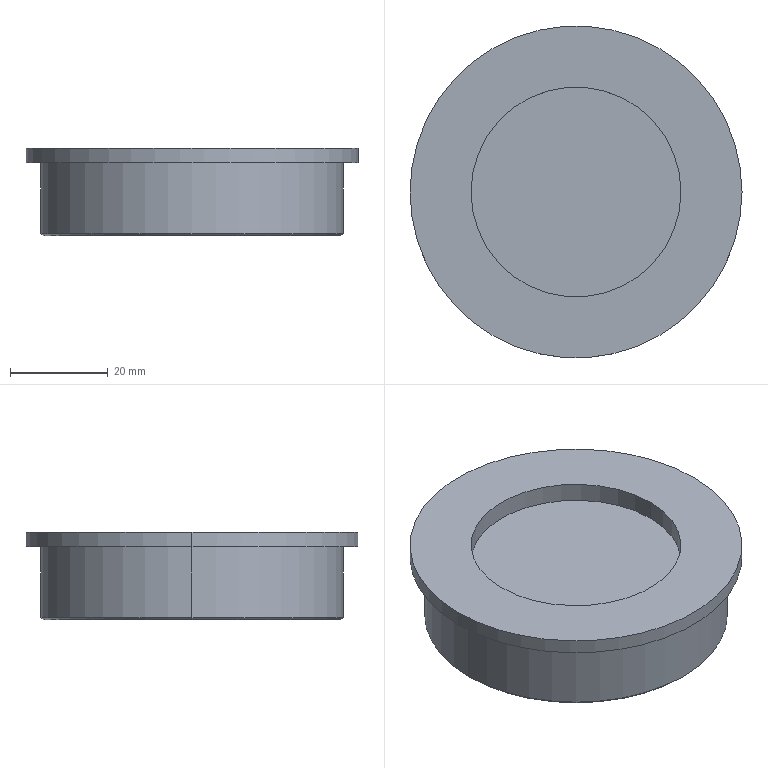Part | SolidWorks | features MBimport 1 | 1 solid | 12 faces | box 68 x 68 x 18 mm | volume 50348 mm3 | cylinder 6 | plane 4 | cone 2 | commonest cylinder face diameters 43 x2 62 x2 68 x2
STEP:
#1=CARTESIAN_POINT('',(-30.5,0.,0.));
#2=VERTEX_POINT('',#1);
#3=CARTESIAN_POINT('',(30.5,0.,0.));
#4=VERTEX_POINT('',#3);
#5=CARTESIAN_POINT('',(0.,0.,0.));
#6=DIRECTION('',(0.,0.,-1.));
#7=DIRECTION('',(-1.,0.,0.));
#8=AXIS2_PLACEMENT_3D('',#5,#6,#7);
#9=CIRCLE('',#8,30.5);
#10=EDGE_CURVE('',#2,#4,#9,.T.);
#11=ORIENTED_EDGE('',*,*,#10,.F.);
#12=CARTESIAN_POINT('',(-31.,0.,0.5));
#13=VERTEX_POINT('',#12);
#14=CARTESIAN_POINT('',(-31.,0.,0.5));
#15=DIRECTION('',(-0.7071,0.,0.7071));
#16=VECTOR('',#15,1000.);
#17=LINE('',#14,#16);
#18=EDGE_CURVE('',#2,#13,#17,.T.);
#19=ORIENTED_EDGE('',*,*,#18,.T.);
#20=CARTESIAN_POINT('',(31.,0.,0.5));
#21=VERTEX_POINT('',#20);
#22=CARTESIAN_POINT('',(0.,0.,0.5));
#23=DIRECTION('',(0.,0.,1.));
#24=DIRECTION('',(-1.,0.,0.));
#25=AXIS2_PLACEMENT_3D('',#22,#23,#24);
#26=CIRCLE('',#25,31.);
#27=EDGE_CURVE('',#21,#13,#26,.T.);
#28=ORIENTED_EDGE('',*,*,#27,.F.);
#29=CARTESIAN_POINT('',(31.,0.,0.5));
#30=DIRECTION('',(0.7071,0.,0.7071));
#31=VECTOR('',#30,1000.);
#32=LINE('',#29,#31);
#33=EDGE_CURVE('',#4,#21,#32,.T.);
#34=ORIENTED_EDGE('',*,*,#33,.F.);
#35=EDGE_LOOP('',(#11,#19,#28,#34));
#36=FACE_OUTER_BOUND('',#35,.T.);
#37=CARTESIAN_POINT('',(0.,0.,0.5));
#38=DIRECTION('',(0.,0.,1.));
#39=DIRECTION('',(1.,0.,0.));
#40=AXIS2_PLACEMENT_3D('',#37,#38,#39);
#41=CONICAL_SURFACE('',#40,31.,0.7854);
#42=ADVANCED_FACE('',(#36),#41,.T.);
#43=CARTESIAN_POINT('',(21.5,0.,14.));
#44=VERTEX_POINT('',#43);
#45=CARTESIAN_POINT('',(-21.5,0.,14.));
#46=VERTEX_POINT('',#45);
#47=CARTESIAN_POINT('',(0.,0.,14.));
#48=DIRECTION('',(0.,0.,-1.));
#49=DIRECTION('',(1.,0.,0.));
#50=AXIS2_PLACEMENT_3D('',#47,#48,#49);
#51=CIRCLE('',#50,21.5);
#52=EDGE_CURVE('',#44,#46,#51,.T.);
#53=ORIENTED_EDGE('',*,*,#52,.T.);
#54=CARTESIAN_POINT('',(-21.5,0.,18.));
#55=VERTEX_POINT('',#54);
#56=CARTESIAN_POINT('',(-21.5,0.,14.));
#57=DIRECTION('',(0.,0.,1.));
#58=VECTOR('',#57,1000.);
#59=LINE('',#56,#58);
#60=EDGE_CURVE('',#46,#55,#59,.T.);
#61=ORIENTED_EDGE('',*,*,#60,.T.);
#62=CARTESIAN_POINT('',(21.5,0.,18.));
#63=VERTEX_POINT('',#62);
#64=CARTESIAN_POINT('',(0.,0.,18.));
#65=DIRECTION('',(0.,0.,1.));
#66=DIRECTION('',(1.,0.,0.));
#67=AXIS2_PLACEMENT_3D('',#64,#65,#66);
#68=CIRCLE('',#67,21.5);
#69=EDGE_CURVE('',#55,#63,#68,.T.);
#70=ORIENTED_EDGE('',*,*,#69,.T.);
#71=CARTESIAN_POINT('',(21.5,0.,14.));
#72=DIRECTION('',(0.,0.,1.));
#73=VECTOR('',#72,1000.);
#74=LINE('',#71,#73);
#75=EDGE_CURVE('',#44,#63,#74,.T.);
#76=ORIENTED_EDGE('',*,*,#75,.F.);
#77=EDGE_LOOP('',(#53,#61,#70,#76));
#78=FACE_OUTER_BOUND('',#77,.T.);
#79=CARTESIAN_POINT('',(0.,0.,14.));
#80=DIRECTION('',(0.,0.,1.));
#81=DIRECTION('',(1.,0.,0.));
#82=AXIS2_PLACEMENT_3D('',#79,#80,#81);
#83=CYLINDRICAL_SURFACE('',#82,21.5);
#84=ADVANCED_FACE('',(#78),#83,.F.);
#85=CARTESIAN_POINT('',(34.,0.,15.));
#86=VERTEX_POINT('',#85);
#87=CARTESIAN_POINT('',(-34.,0.,15.));
#88=VERTEX_POINT('',#87);
#89=CARTESIAN_POINT('',(0.,0.,15.));
#90=DIRECTION('',(0.,0.,1.));
#91=DIRECTION('',(1.,0.,0.));
#92=AXIS2_PLACEMENT_3D('',#89,#90,#91);
#93=CIRCLE('',#92,34.);
#94=EDGE_CURVE('',#86,#88,#93,.T.);
#95=ORIENTED_EDGE('',*,*,#94,.T.);
#96=CARTESIAN_POINT('',(-34.,0.,18.));
#97=VERTEX_POINT('',#96);
#98=CARTESIAN_POINT('',(-34.,0.,15.));
#99=DIRECTION('',(0.,0.,1.));
#100=VECTOR('',#99,1000.);
#101=LINE('',#98,#100);
#102=EDGE_CURVE('',#88,#97,#101,.T.);
#103=ORIENTED_EDGE('',*,*,#102,.T.);
#104=CARTESIAN_POINT('',(34.,0.,18.));
#105=VERTEX_POINT('',#104);
#106=CARTESIAN_POINT('',(0.,0.,18.));
#107=DIRECTION('',(0.,0.,-1.));
#108=DIRECTION('',(1.,0.,0.));
#109=AXIS2_PLACEMENT_3D('',#106,#107,#108);
#110=CIRCLE('',#109,34.);
#111=EDGE_CURVE('',#97,#105,#110,.T.);
#112=ORIENTED_EDGE('',*,*,#111,.T.);
#113=CARTESIAN_POINT('',(34.,0.,15.));
#114=DIRECTION('',(0.,0.,1.));
#115=VECTOR('',#114,1000.);
#116=LINE('',#113,#115);
#117=EDGE_CURVE('',#86,#105,#116,.T.);
#118=ORIENTED_EDGE('',*,*,#117,.F.);
#119=EDGE_LOOP('',(#95,#103,#112,#118));
#120=FACE_OUTER_BOUND('',#119,.T.);
#121=CARTESIAN_POINT('',(0.,0.,15.));
#122=DIRECTION('',(0.,0.,1.));
#123=DIRECTION('',(1.,0.,0.));
#124=AXIS2_PLACEMENT_3D('',#121,#122,#123);
#125=CYLINDRICAL_SURFACE('',#124,34.);
#126=ADVANCED_FACE('',(#120),#125,.T.);
#127=ORIENTED_EDGE('',*,*,#27,.T.);
#128=CARTESIAN_POINT('',(-31.,0.,15.));
#129=VERTEX_POINT('',#128);
#130=CARTESIAN_POINT('',(-31.,0.,0.));
#131=DIRECTION('',(0.,0.,1.));
#132=VECTOR('',#131,1000.);
#133=LINE('',#130,#132);
#134=EDGE_CURVE('',#13,#129,#133,.T.);
#135=ORIENTED_EDGE('',*,*,#134,.T.);
#136=CARTESIAN_POINT('',(31.,0.,15.));
#137=VERTEX_POINT('',#136);
#138=CARTESIAN_POINT('',(0.,0.,15.));
#139=DIRECTION('',(0.,0.,-1.));
#140=DIRECTION('',(1.,0.,0.));
#141=AXIS2_PLACEMENT_3D('',#138,#139,#140);
#142=CIRCLE('',#141,31.);
#143=EDGE_CURVE('',#129,#137,#142,.T.);
#144=ORIENTED_EDGE('',*,*,#143,.T.);
#145=CARTESIAN_POINT('',(31.,0.,0.));
#146=DIRECTION('',(0.,0.,1.));
#147=VECTOR('',#146,1000.);
#148=LINE('',#145,#147);
#149=EDGE_CURVE('',#21,#137,#148,.T.);
#150=ORIENTED_EDGE('',*,*,#149,.F.);
#151=EDGE_LOOP('',(#127,#135,#144,#150));
#152=FACE_OUTER_BOUND('',#151,.T.);
#153=CARTESIAN_POINT('',(0.,0.,0.));
#154=DIRECTION('',(0.,0.,1.));
#155=DIRECTION('',(1.,0.,0.));
#156=AXIS2_PLACEMENT_3D('',#153,#154,#155);
#157=CYLINDRICAL_SURFACE('',#156,31.);
#158=ADVANCED_FACE('',(#152),#157,.T.);
#159=CARTESIAN_POINT('',(0.,0.,0.));
#160=DIRECTION('',(0.,0.,-1.));
#161=DIRECTION('',(-1.,0.,0.));
#162=AXIS2_PLACEMENT_3D('',#159,#160,#161);
#163=CIRCLE('',#162,30.5);
#164=EDGE_CURVE('',#4,#2,#163,.T.);
#165=ORIENTED_EDGE('',*,*,#164,.T.);
#166=ORIENTED_EDGE('',*,*,#10,.T.);
#167=EDGE_LOOP('',(#165,#166));
#168=FACE_OUTER_BOUND('',#167,.T.);
#169=CARTESIAN_POINT('',(0.,0.,0.));
#170=DIRECTION('',(0.,0.,-1.));
#171=DIRECTION('',(0.,-1.,0.));
#172=AXIS2_PLACEMENT_3D('',#169,#170,#171);
#173=PLANE('',#172);
#174=ADVANCED_FACE('',(#168),#173,.T.);
#175=ORIENTED_EDGE('',*,*,#134,.F.);
#176=CARTESIAN_POINT('',(0.,0.,0.5));
#177=DIRECTION('',(0.,0.,1.));
#178=DIRECTION('',(-1.,0.,0.));
#179=AXIS2_PLACEMENT_3D('',#176,#177,#178);
#180=CIRCLE('',#179,31.);
#181=EDGE_CURVE('',#13,#21,#180,.T.);
#182=ORIENTED_EDGE('',*,*,#181,.T.);
#183=ORIENTED_EDGE('',*,*,#149,.T.);
#184=CARTESIAN_POINT('',(0.,0.,15.));
#185=DIRECTION('',(0.,0.,-1.));
#186=DIRECTION('',(1.,0.,0.));
#187=AXIS2_PLACEMENT_3D('',#184,#185,#186);
#188=CIRCLE('',#187,31.);
#189=EDGE_CURVE('',#137,#129,#188,.T.);
#190=ORIENTED_EDGE('',*,*,#189,.T.);
#191=EDGE_LOOP('',(#175,#182,#183,#190));
#192=FACE_OUTER_BOUND('',#191,.T.);
#193=CARTESIAN_POINT('',(0.,0.,0.));
#194=DIRECTION('',(0.,0.,1.));
#195=DIRECTION('',(1.,0.,0.));
#196=AXIS2_PLACEMENT_3D('',#193,#194,#195);
#197=CYLINDRICAL_SURFACE('',#196,31.);
#198=ADVANCED_FACE('',(#192),#197,.T.);
#199=CARTESIAN_POINT('',(0.,0.,18.));
#200=DIRECTION('',(0.,0.,1.));
#201=DIRECTION('',(1.,0.,0.));
#202=AXIS2_PLACEMENT_3D('',#199,#200,#201);
#203=CIRCLE('',#202,21.5);
#204=EDGE_CURVE('',#63,#55,#203,.T.);
#205=ORIENTED_EDGE('',*,*,#204,.F.);
#206=ORIENTED_EDGE('',*,*,#69,.F.);
#207=EDGE_LOOP('',(#205,#206));
#208=FACE_BOUND('',#207,.T.);
#209=CARTESIAN_POINT('',(0.,0.,18.));
#210=DIRECTION('',(0.,0.,-1.));
#211=DIRECTION('',(1.,0.,0.));
#212=AXIS2_PLACEMENT_3D('',#209,#210,#211);
#213=CIRCLE('',#212,34.);
#214=EDGE_CURVE('',#105,#97,#213,.T.);
#215=ORIENTED_EDGE('',*,*,#214,.F.);
#216=ORIENTED_EDGE('',*,*,#111,.F.);
#217=EDGE_LOOP('',(#215,#216));
#218=FACE_OUTER_BOUND('',#217,.T.);
#219=CARTESIAN_POINT('',(0.,0.,18.));
#220=DIRECTION('',(0.,0.,1.));
#221=DIRECTION('',(1.,0.,0.));
#222=AXIS2_PLACEMENT_3D('',#219,#220,#221);
#223=PLANE('',#222);
#224=ADVANCED_FACE('',(#208,#218),#223,.T.);
#225=ORIENTED_EDGE('',*,*,#189,.F.);
#226=ORIENTED_EDGE('',*,*,#143,.F.);
#227=EDGE_LOOP('',(#225,#226));
#228=FACE_BOUND('',#227,.T.);
#229=ORIENTED_EDGE('',*,*,#94,.F.);
#230=CARTESIAN_POINT('',(0.,0.,15.));
#231=DIRECTION('',(0.,0.,1.));
#232=DIRECTION('',(1.,0.,0.));
#233=AXIS2_PLACEMENT_3D('',#230,#231,#232);
#234=CIRCLE('',#233,34.);
#235=EDGE_CURVE('',#88,#86,#234,.T.);
#236=ORIENTED_EDGE('',*,*,#235,.F.);
#237=EDGE_LOOP('',(#229,#236));
#238=FACE_OUTER_BOUND('',#237,.T.);
#239=CARTESIAN_POINT('',(0.,0.,15.));
#240=DIRECTION('',(0.,0.,-1.));
#241=DIRECTION('',(0.,-1.,0.));
#242=AXIS2_PLACEMENT_3D('',#239,#240,#241);
#243=PLANE('',#242);
#244=ADVANCED_FACE('',(#228,#238),#243,.T.);
#245=ORIENTED_EDGE('',*,*,#102,.F.);
#246=ORIENTED_EDGE('',*,*,#235,.T.);
#247=ORIENTED_EDGE('',*,*,#117,.T.);
#248=ORIENTED_EDGE('',*,*,#214,.T.);
#249=EDGE_LOOP('',(#245,#246,#247,#248));
#250=FACE_OUTER_BOUND('',#249,.T.);
#251=CARTESIAN_POINT('',(0.,0.,15.));
#252=DIRECTION('',(0.,0.,1.));
#253=DIRECTION('',(1.,0.,0.));
#254=AXIS2_PLACEMENT_3D('',#251,#252,#253);
#255=CYLINDRICAL_SURFACE('',#254,34.);
#256=ADVANCED_FACE('',(#250),#255,.T.);
#257=ORIENTED_EDGE('',*,*,#60,.F.);
#258=CARTESIAN_POINT('',(0.,0.,14.));
#259=DIRECTION('',(0.,0.,-1.));
#260=DIRECTION('',(1.,0.,0.));
#261=AXIS2_PLACEMENT_3D('',#258,#259,#260);
#262=CIRCLE('',#261,21.5);
#263=EDGE_CURVE('',#46,#44,#262,.T.);
#264=ORIENTED_EDGE('',*,*,#263,.T.);
#265=ORIENTED_EDGE('',*,*,#75,.T.);
#266=ORIENTED_EDGE('',*,*,#204,.T.);
#267=EDGE_LOOP('',(#257,#264,#265,#266));
#268=FACE_OUTER_BOUND('',#267,.T.);
#269=CARTESIAN_POINT('',(0.,0.,14.));
#270=DIRECTION('',(0.,0.,1.));
#271=DIRECTION('',(1.,0.,0.));
#272=AXIS2_PLACEMENT_3D('',#269,#270,#271);
#273=CYLINDRICAL_SURFACE('',#272,21.5);
#274=ADVANCED_FACE('',(#268),#273,.F.);
#275=ORIENTED_EDGE('',*,*,#52,.F.);
#276=ORIENTED_EDGE('',*,*,#263,.F.);
#277=EDGE_LOOP('',(#275,#276));
#278=FACE_OUTER_BOUND('',#277,.T.);
#279=CARTESIAN_POINT('',(0.,0.,14.));
#280=DIRECTION('',(0.,0.,1.));
#281=DIRECTION('',(1.,0.,0.));
#282=AXIS2_PLACEMENT_3D('',#279,#280,#281);
#283=PLANE('',#282);
#284=ADVANCED_FACE('',(#278),#283,.T.);
#285=ORIENTED_EDGE('',*,*,#18,.F.);
#286=ORIENTED_EDGE('',*,*,#164,.F.);
#287=ORIENTED_EDGE('',*,*,#33,.T.);
#288=ORIENTED_EDGE('',*,*,#181,.F.);
#289=EDGE_LOOP('',(#285,#286,#287,#288));
#290=FACE_OUTER_BOUND('',#289,.T.);
#291=CARTESIAN_POINT('',(0.,0.,0.5));
#292=DIRECTION('',(0.,0.,1.));
#293=DIRECTION('',(1.,0.,0.));
#294=AXIS2_PLACEMENT_3D('',#291,#292,#293);
#295=CONICAL_SURFACE('',#294,31.,0.7854);
#296=ADVANCED_FACE('',(#290),#295,.T.);
#297=CLOSED_SHELL('',(#42,#84,#126,#158,#174,#198,#224,#244,#256,#274,#284,#296));
#298=MANIFOLD_SOLID_BREP('',#297);
#299=CARTESIAN_POINT('',(0.,0.,0.));
#300=DIRECTION('',(0.,0.,1.));
#301=DIRECTION('',(1.,0.,0.));
#302=AXIS2_PLACEMENT_3D('',#299,#300,#301);
#303=(LENGTH_UNIT()NAMED_UNIT(*)SI_UNIT(.MILLI.,.METRE.));
#304=UNCERTAINTY_MEASURE_WITH_UNIT(LENGTH_MEASURE(0.00001),#303,'','');
#305=(NAMED_UNIT(*)PLANE_ANGLE_UNIT()SI_UNIT($,.RADIAN.));
#306=(NAMED_UNIT(*)SI_UNIT($,.STERADIAN.)SOLID_ANGLE_UNIT());
#307=(GEOMETRIC_REPRESENTATION_CONTEXT(3)GLOBAL_UNCERTAINTY_ASSIGNED_CONTEXT((#304))GLOBAL_UNIT_ASSIGNED_CONTEXT((#303,#305,#306))REPRESENTATION_CONTEXT('',''));
#308=ADVANCED_BREP_SHAPE_REPRESENTATION('',(#298,#302),#307);